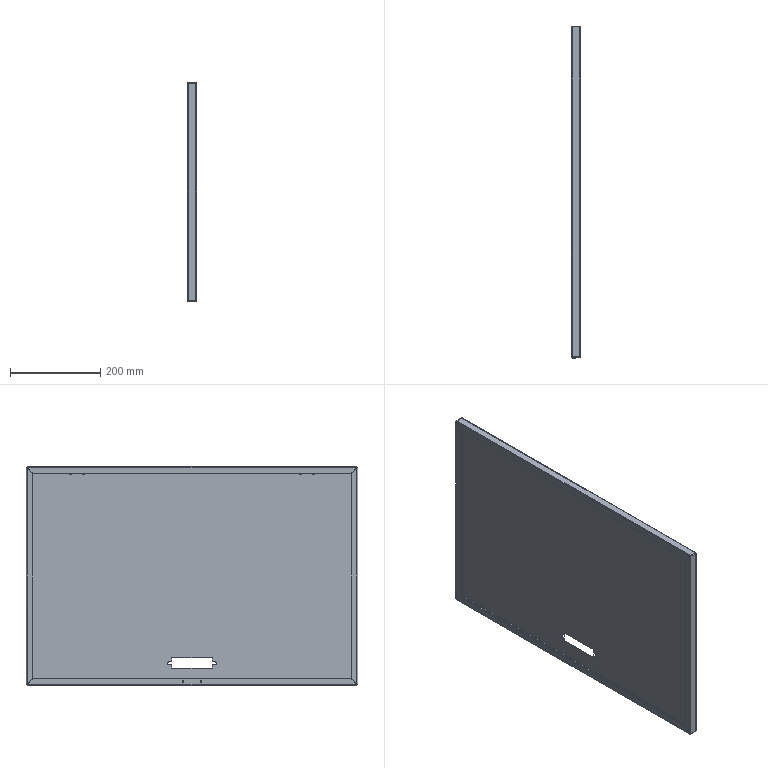Part | STEP file | JBJ-P-1000-17 | 1 solid | 88 faces | box 20 x 735 x 485 mm | volume 514895 mm3 | plane 48 | cylinder 24 | spline 16 | commonest cylinder face diameters 2 x8 4.4 x8 6.5 x4 4 x2 7 x2